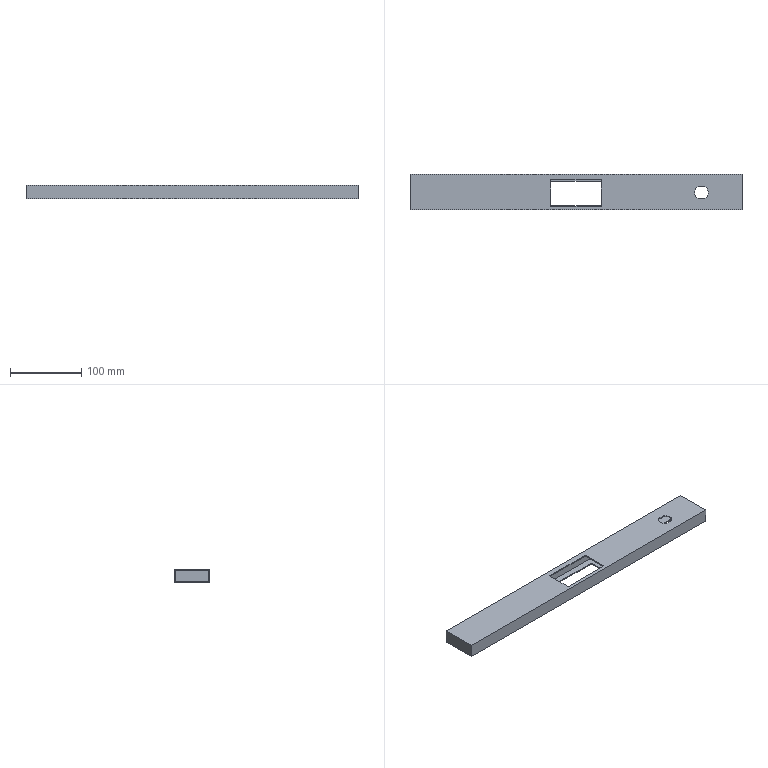Part | SolidWorks | features ICE 4, Extrusion 1, Shell 1 | 1 solid | 30 faces | box 466 x 50 x 19 mm | volume 83409 mm3 | plane 24 | cylinder 6 | commonest cylinder face diameters 19 x3 60 x3
STEP:
#1=CARTESIAN_POINT('',(379.,24.,1.5));
#2=VERTEX_POINT('',#1);
#3=CARTESIAN_POINT('',(381.728,36.5,1.5));
#4=VERTEX_POINT('',#3);
#5=CARTESIAN_POINT('',(409.,24.,1.5));
#6=DIRECTION('',(0.,0.,-1.));
#7=DIRECTION('',(-1.,0.,0.));
#8=AXIS2_PLACEMENT_3D('',#5,#6,#7);
#9=CIRCLE('',#8,30.);
#10=EDGE_CURVE('',#2,#4,#9,.T.);
#11=ORIENTED_EDGE('',*,*,#10,.F.);
#12=CARTESIAN_POINT('',(379.,24.,0.));
#13=VERTEX_POINT('',#12);
#14=CARTESIAN_POINT('',(379.,24.,2.));
#15=DIRECTION('',(0.,0.,-1.));
#16=VECTOR('',#15,1000.);
#17=LINE('',#14,#16);
#18=EDGE_CURVE('',#2,#13,#17,.T.);
#19=ORIENTED_EDGE('',*,*,#18,.T.);
#20=CARTESIAN_POINT('',(381.728,36.5,0.));
#21=VERTEX_POINT('',#20);
#22=CARTESIAN_POINT('',(409.,24.,0.));
#23=DIRECTION('',(0.,0.,-1.));
#24=DIRECTION('',(-1.,0.,0.));
#25=AXIS2_PLACEMENT_3D('',#22,#23,#24);
#26=CIRCLE('',#25,30.);
#27=EDGE_CURVE('',#13,#21,#26,.T.);
#28=ORIENTED_EDGE('',*,*,#27,.T.);
#29=CARTESIAN_POINT('',(381.728,36.5,2.));
#30=DIRECTION('',(0.,0.,-1.));
#31=VECTOR('',#30,1000.);
#32=LINE('',#29,#31);
#33=EDGE_CURVE('',#4,#21,#32,.T.);
#34=ORIENTED_EDGE('',*,*,#33,.F.);
#35=EDGE_LOOP('',(#11,#19,#28,#34));
#36=FACE_OUTER_BOUND('',#35,.T.);
#37=CARTESIAN_POINT('',(409.,24.,2.));
#38=DIRECTION('',(0.,0.,-1.));
#39=DIRECTION('',(-1.,0.,0.));
#40=AXIS2_PLACEMENT_3D('',#37,#38,#39);
#41=CYLINDRICAL_SURFACE('',#40,30.);
#42=ADVANCED_FACE('',(#36),#41,.F.);
#43=CARTESIAN_POINT('',(399.5,24.,19.));
#44=VERTEX_POINT('',#43);
#45=CARTESIAN_POINT('',(404.29,32.25,19.));
#46=VERTEX_POINT('',#45);
#47=CARTESIAN_POINT('',(409.,24.,19.));
#48=DIRECTION('',(0.,0.,-1.));
#49=DIRECTION('',(-1.,0.,0.));
#50=AXIS2_PLACEMENT_3D('',#47,#48,#49);
#51=CIRCLE('',#50,9.5);
#52=EDGE_CURVE('',#44,#46,#51,.T.);
#53=ORIENTED_EDGE('',*,*,#52,.F.);
#54=CARTESIAN_POINT('',(399.5,24.,17.5));
#55=VERTEX_POINT('',#54);
#56=CARTESIAN_POINT('',(399.5,24.,19.));
#57=DIRECTION('',(0.,0.,-1.));
#58=VECTOR('',#57,1000.);
#59=LINE('',#56,#58);
#60=EDGE_CURVE('',#44,#55,#59,.T.);
#61=ORIENTED_EDGE('',*,*,#60,.T.);
#62=CARTESIAN_POINT('',(404.29,32.25,17.5));
#63=VERTEX_POINT('',#62);
#64=CARTESIAN_POINT('',(409.,24.,17.5));
#65=DIRECTION('',(0.,0.,-1.));
#66=DIRECTION('',(-1.,0.,0.));
#67=AXIS2_PLACEMENT_3D('',#64,#65,#66);
#68=CIRCLE('',#67,9.5);
#69=EDGE_CURVE('',#55,#63,#68,.T.);
#70=ORIENTED_EDGE('',*,*,#69,.T.);
#71=CARTESIAN_POINT('',(404.29,32.25,19.));
#72=DIRECTION('',(0.,0.,-1.));
#73=VECTOR('',#72,1000.);
#74=LINE('',#71,#73);
#75=EDGE_CURVE('',#46,#63,#74,.T.);
#76=ORIENTED_EDGE('',*,*,#75,.F.);
#77=EDGE_LOOP('',(#53,#61,#70,#76));
#78=FACE_OUTER_BOUND('',#77,.T.);
#79=CARTESIAN_POINT('',(409.,24.,19.));
#80=DIRECTION('',(0.,0.,-1.));
#81=DIRECTION('',(-1.,0.,0.));
#82=AXIS2_PLACEMENT_3D('',#79,#80,#81);
#83=CYLINDRICAL_SURFACE('',#82,9.5);
#84=ADVANCED_FACE('',(#78),#83,.F.);
#85=CARTESIAN_POINT('',(0.,50.,0.));
#86=VERTEX_POINT('',#85);
#87=CARTESIAN_POINT('',(0.,0.,0.));
#88=VERTEX_POINT('',#87);
#89=CARTESIAN_POINT('',(0.,0.,0.));
#90=DIRECTION('',(0.,-1.,0.));
#91=VECTOR('',#90,1000.);
#92=LINE('',#89,#91);
#93=EDGE_CURVE('',#86,#88,#92,.T.);
#94=ORIENTED_EDGE('',*,*,#93,.T.);
#95=CARTESIAN_POINT('',(0.,0.,19.));
#96=VERTEX_POINT('',#95);
#97=CARTESIAN_POINT('',(0.,0.,19.));
#98=DIRECTION('',(0.,0.,-1.));
#99=VECTOR('',#98,1000.);
#100=LINE('',#97,#99);
#101=EDGE_CURVE('',#96,#88,#100,.T.);
#102=ORIENTED_EDGE('',*,*,#101,.F.);
#103=CARTESIAN_POINT('',(0.,50.,19.));
#104=VERTEX_POINT('',#103);
#105=CARTESIAN_POINT('',(0.,0.,19.));
#106=DIRECTION('',(0.,-1.,0.));
#107=VECTOR('',#106,1000.);
#108=LINE('',#105,#107);
#109=EDGE_CURVE('',#104,#96,#108,.T.);
#110=ORIENTED_EDGE('',*,*,#109,.F.);
#111=CARTESIAN_POINT('',(0.,50.,19.));
#112=DIRECTION('',(0.,0.,-1.));
#113=VECTOR('',#112,1000.);
#114=LINE('',#111,#113);
#115=EDGE_CURVE('',#104,#86,#114,.T.);
#116=ORIENTED_EDGE('',*,*,#115,.T.);
#117=EDGE_LOOP('',(#94,#102,#110,#116));
#118=FACE_OUTER_BOUND('',#117,.T.);
#119=CARTESIAN_POINT('',(0.,0.,19.));
#120=DIRECTION('',(1.,0.,0.));
#121=DIRECTION('',(0.,0.,-1.));
#122=AXIS2_PLACEMENT_3D('',#119,#120,#121);
#123=PLANE('',#122);
#124=ADVANCED_FACE('',(#118),#123,.F.);
#125=CARTESIAN_POINT('',(466.,0.,0.));
#126=VERTEX_POINT('',#125);
#127=CARTESIAN_POINT('',(0.,0.,0.));
#128=DIRECTION('',(1.,0.,0.));
#129=VECTOR('',#128,1000.);
#130=LINE('',#127,#129);
#131=EDGE_CURVE('',#88,#126,#130,.T.);
#132=ORIENTED_EDGE('',*,*,#131,.T.);
#133=CARTESIAN_POINT('',(466.,0.,19.));
#134=VERTEX_POINT('',#133);
#135=CARTESIAN_POINT('',(466.,0.,19.));
#136=DIRECTION('',(0.,0.,-1.));
#137=VECTOR('',#136,1000.);
#138=LINE('',#135,#137);
#139=EDGE_CURVE('',#134,#126,#138,.T.);
#140=ORIENTED_EDGE('',*,*,#139,.F.);
#141=CARTESIAN_POINT('',(0.,0.,19.));
#142=DIRECTION('',(1.,0.,0.));
#143=VECTOR('',#142,1000.);
#144=LINE('',#141,#143);
#145=EDGE_CURVE('',#96,#134,#144,.T.);
#146=ORIENTED_EDGE('',*,*,#145,.F.);
#147=ORIENTED_EDGE('',*,*,#101,.T.);
#148=EDGE_LOOP('',(#132,#140,#146,#147));
#149=FACE_OUTER_BOUND('',#148,.T.);
#150=CARTESIAN_POINT('',(0.,0.,19.));
#151=DIRECTION('',(0.,1.,0.));
#152=DIRECTION('',(0.,0.,1.));
#153=AXIS2_PLACEMENT_3D('',#150,#151,#152);
#154=PLANE('',#153);
#155=ADVANCED_FACE('',(#149),#154,.F.);
#156=CARTESIAN_POINT('',(466.,50.,0.));
#157=VERTEX_POINT('',#156);
#158=CARTESIAN_POINT('',(466.,0.,0.));
#159=DIRECTION('',(0.,1.,0.));
#160=VECTOR('',#159,1000.);
#161=LINE('',#158,#160);
#162=EDGE_CURVE('',#126,#157,#161,.T.);
#163=ORIENTED_EDGE('',*,*,#162,.T.);
#164=CARTESIAN_POINT('',(466.,50.,19.));
#165=VERTEX_POINT('',#164);
#166=CARTESIAN_POINT('',(466.,50.,19.));
#167=DIRECTION('',(0.,0.,-1.));
#168=VECTOR('',#167,1000.);
#169=LINE('',#166,#168);
#170=EDGE_CURVE('',#165,#157,#169,.T.);
#171=ORIENTED_EDGE('',*,*,#170,.F.);
#172=CARTESIAN_POINT('',(466.,0.,19.));
#173=DIRECTION('',(0.,1.,0.));
#174=VECTOR('',#173,1000.);
#175=LINE('',#172,#174);
#176=EDGE_CURVE('',#134,#165,#175,.T.);
#177=ORIENTED_EDGE('',*,*,#176,.F.);
#178=ORIENTED_EDGE('',*,*,#139,.T.);
#179=EDGE_LOOP('',(#163,#171,#177,#178));
#180=FACE_OUTER_BOUND('',#179,.T.);
#181=CARTESIAN_POINT('',(466.,0.,19.));
#182=DIRECTION('',(-1.,0.,0.));
#183=DIRECTION('',(0.,0.,1.));
#184=AXIS2_PLACEMENT_3D('',#181,#182,#183);
#185=PLANE('',#184);
#186=ADVANCED_FACE('',(#180),#185,.F.);
#187=CARTESIAN_POINT('',(0.,50.,0.));
#188=DIRECTION('',(-1.,0.,0.));
#189=VECTOR('',#188,1000.);
#190=LINE('',#187,#189);
#191=EDGE_CURVE('',#157,#86,#190,.T.);
#192=ORIENTED_EDGE('',*,*,#191,.T.);
#193=ORIENTED_EDGE('',*,*,#115,.F.);
#194=CARTESIAN_POINT('',(0.,50.,19.));
#195=DIRECTION('',(-1.,0.,0.));
#196=VECTOR('',#195,1000.);
#197=LINE('',#194,#196);
#198=EDGE_CURVE('',#165,#104,#197,.T.);
#199=ORIENTED_EDGE('',*,*,#198,.F.);
#200=ORIENTED_EDGE('',*,*,#170,.T.);
#201=EDGE_LOOP('',(#192,#193,#199,#200));
#202=FACE_OUTER_BOUND('',#201,.T.);
#203=CARTESIAN_POINT('',(0.,50.,19.));
#204=DIRECTION('',(0.,-1.,0.));
#205=DIRECTION('',(0.,0.,-1.));
#206=AXIS2_PLACEMENT_3D('',#203,#204,#205);
#207=PLANE('',#206);
#208=ADVANCED_FACE('',(#202),#207,.F.);
#209=CARTESIAN_POINT('',(413.71,32.25,19.));
#210=VERTEX_POINT('',#209);
#211=CARTESIAN_POINT('',(413.71,32.25,19.));
#212=DIRECTION('',(1.,0.,0.));
#213=VECTOR('',#212,1000.);
#214=LINE('',#211,#213);
#215=EDGE_CURVE('',#46,#210,#214,.T.);
#216=ORIENTED_EDGE('',*,*,#215,.T.);
#217=CARTESIAN_POINT('',(413.71,15.75,19.));
#218=VERTEX_POINT('',#217);
#219=CARTESIAN_POINT('',(409.,24.,19.));
#220=DIRECTION('',(0.,0.,-1.));
#221=DIRECTION('',(-1.,0.,0.));
#222=AXIS2_PLACEMENT_3D('',#219,#220,#221);
#223=CIRCLE('',#222,9.5);
#224=EDGE_CURVE('',#210,#218,#223,.T.);
#225=ORIENTED_EDGE('',*,*,#224,.T.);
#226=CARTESIAN_POINT('',(404.29,15.75,19.));
#227=VERTEX_POINT('',#226);
#228=CARTESIAN_POINT('',(413.71,15.75,19.));
#229=DIRECTION('',(-1.,0.,0.));
#230=VECTOR('',#229,1000.);
#231=LINE('',#228,#230);
#232=EDGE_CURVE('',#218,#227,#231,.T.);
#233=ORIENTED_EDGE('',*,*,#232,.T.);
#234=CARTESIAN_POINT('',(409.,24.,19.));
#235=DIRECTION('',(0.,0.,-1.));
#236=DIRECTION('',(-1.,0.,0.));
#237=AXIS2_PLACEMENT_3D('',#234,#235,#236);
#238=CIRCLE('',#237,9.5);
#239=EDGE_CURVE('',#227,#44,#238,.T.);
#240=ORIENTED_EDGE('',*,*,#239,.T.);
#241=ORIENTED_EDGE('',*,*,#52,.T.);
#242=EDGE_LOOP('',(#216,#225,#233,#240,#241));
#243=FACE_BOUND('',#242,.T.);
#244=CARTESIAN_POINT('',(197.5,5.,19.));
#245=VERTEX_POINT('',#244);
#246=CARTESIAN_POINT('',(268.5,5.,19.));
#247=VERTEX_POINT('',#246);
#248=CARTESIAN_POINT('',(197.5,5.,19.));
#249=DIRECTION('',(1.,0.,0.));
#250=VECTOR('',#249,1000.);
#251=LINE('',#248,#250);
#252=EDGE_CURVE('',#245,#247,#251,.T.);
#253=ORIENTED_EDGE('',*,*,#252,.F.);
#254=CARTESIAN_POINT('',(197.5,42.,19.));
#255=VERTEX_POINT('',#254);
#256=CARTESIAN_POINT('',(197.5,5.,19.));
#257=DIRECTION('',(0.,-1.,0.));
#258=VECTOR('',#257,1000.);
#259=LINE('',#256,#258);
#260=EDGE_CURVE('',#255,#245,#259,.T.);
#261=ORIENTED_EDGE('',*,*,#260,.F.);
#262=CARTESIAN_POINT('',(268.5,42.,19.));
#263=VERTEX_POINT('',#262);
#264=CARTESIAN_POINT('',(197.5,42.,19.));
#265=DIRECTION('',(-1.,0.,0.));
#266=VECTOR('',#265,1000.);
#267=LINE('',#264,#266);
#268=EDGE_CURVE('',#263,#255,#267,.T.);
#269=ORIENTED_EDGE('',*,*,#268,.F.);
#270=CARTESIAN_POINT('',(268.5,5.,19.));
#271=DIRECTION('',(0.,1.,0.));
#272=VECTOR('',#271,1000.);
#273=LINE('',#270,#272);
#274=EDGE_CURVE('',#247,#263,#273,.T.);
#275=ORIENTED_EDGE('',*,*,#274,.F.);
#276=EDGE_LOOP('',(#253,#261,#269,#275));
#277=FACE_BOUND('',#276,.T.);
#278=ORIENTED_EDGE('',*,*,#109,.T.);
#279=ORIENTED_EDGE('',*,*,#145,.T.);
#280=ORIENTED_EDGE('',*,*,#176,.T.);
#281=ORIENTED_EDGE('',*,*,#198,.T.);
#282=EDGE_LOOP('',(#278,#279,#280,#281));
#283=FACE_OUTER_BOUND('',#282,.T.);
#284=CARTESIAN_POINT('',(0.,50.,19.));
#285=DIRECTION('',(0.,0.,-1.));
#286=DIRECTION('',(-1.,0.,0.));
#287=AXIS2_PLACEMENT_3D('',#284,#285,#286);
#288=PLANE('',#287);
#289=ADVANCED_FACE('',(#243,#277,#283),#288,.F.);
#290=CARTESIAN_POINT('',(381.728,11.5,0.));
#291=VERTEX_POINT('',#290);
#292=CARTESIAN_POINT('',(409.,24.,0.));
#293=DIRECTION('',(0.,0.,-1.));
#294=DIRECTION('',(-1.,0.,0.));
#295=AXIS2_PLACEMENT_3D('',#292,#293,#294);
#296=CIRCLE('',#295,30.);
#297=EDGE_CURVE('',#291,#13,#296,.T.);
#298=ORIENTED_EDGE('',*,*,#297,.F.);
#299=CARTESIAN_POINT('',(436.272,11.5,0.));
#300=VERTEX_POINT('',#299);
#301=CARTESIAN_POINT('',(436.272,11.5,0.));
#302=DIRECTION('',(-1.,0.,0.));
#303=VECTOR('',#302,1000.);
#304=LINE('',#301,#303);
#305=EDGE_CURVE('',#300,#291,#304,.T.);
#306=ORIENTED_EDGE('',*,*,#305,.F.);
#307=CARTESIAN_POINT('',(436.272,36.5,0.));
#308=VERTEX_POINT('',#307);
#309=CARTESIAN_POINT('',(409.,24.,0.));
#310=DIRECTION('',(0.,0.,-1.));
#311=DIRECTION('',(-1.,0.,0.));
#312=AXIS2_PLACEMENT_3D('',#309,#310,#311);
#313=CIRCLE('',#312,30.);
#314=EDGE_CURVE('',#308,#300,#313,.T.);
#315=ORIENTED_EDGE('',*,*,#314,.F.);
#316=CARTESIAN_POINT('',(436.272,36.5,0.));
#317=DIRECTION('',(1.,0.,0.));
#318=VECTOR('',#317,1000.);
#319=LINE('',#316,#318);
#320=EDGE_CURVE('',#21,#308,#319,.T.);
#321=ORIENTED_EDGE('',*,*,#320,.F.);
#322=ORIENTED_EDGE('',*,*,#27,.F.);
#323=EDGE_LOOP('',(#298,#306,#315,#321,#322));
#324=FACE_BOUND('',#323,.T.);
#325=CARTESIAN_POINT('',(278.,40.,0.));
#326=VERTEX_POINT('',#325);
#327=CARTESIAN_POINT('',(278.,6.,0.));
#328=VERTEX_POINT('',#327);
#329=CARTESIAN_POINT('',(278.,6.,0.));
#330=DIRECTION('',(0.,-1.,0.));
#331=VECTOR('',#330,1000.);
#332=LINE('',#329,#331);
#333=EDGE_CURVE('',#326,#328,#332,.T.);
#334=ORIENTED_EDGE('',*,*,#333,.F.);
#335=CARTESIAN_POINT('',(188.,40.,0.));
#336=VERTEX_POINT('',#335);
#337=CARTESIAN_POINT('',(278.,40.,0.));
#338=DIRECTION('',(1.,0.,0.));
#339=VECTOR('',#338,1000.);
#340=LINE('',#337,#339);
#341=EDGE_CURVE('',#336,#326,#340,.T.);
#342=ORIENTED_EDGE('',*,*,#341,.F.);
#343=CARTESIAN_POINT('',(188.,6.,0.));
#344=VERTEX_POINT('',#343);
#345=CARTESIAN_POINT('',(188.,6.,0.));
#346=DIRECTION('',(0.,1.,0.));
#347=VECTOR('',#346,1000.);
#348=LINE('',#345,#347);
#349=EDGE_CURVE('',#344,#336,#348,.T.);
#350=ORIENTED_EDGE('',*,*,#349,.F.);
#351=CARTESIAN_POINT('',(278.,6.,0.));
#352=DIRECTION('',(-1.,0.,0.));
#353=VECTOR('',#352,1000.);
#354=LINE('',#351,#353);
#355=EDGE_CURVE('',#328,#344,#354,.T.);
#356=ORIENTED_EDGE('',*,*,#355,.F.);
#357=EDGE_LOOP('',(#334,#342,#350,#356));
#358=FACE_BOUND('',#357,.T.);
#359=ORIENTED_EDGE('',*,*,#93,.F.);
#360=ORIENTED_EDGE('',*,*,#191,.F.);
#361=ORIENTED_EDGE('',*,*,#162,.F.);
#362=ORIENTED_EDGE('',*,*,#131,.F.);
#363=EDGE_LOOP('',(#359,#360,#361,#362));
#364=FACE_OUTER_BOUND('',#363,.T.);
#365=CARTESIAN_POINT('',(0.,50.,0.));
#366=DIRECTION('',(0.,0.,-1.));
#367=DIRECTION('',(-1.,0.,0.));
#368=AXIS2_PLACEMENT_3D('',#365,#366,#367);
#369=PLANE('',#368);
#370=ADVANCED_FACE('',(#324,#358,#364),#369,.T.);
#371=ORIENTED_EDGE('',*,*,#260,.T.);
#372=CARTESIAN_POINT('',(197.5,5.,17.5));
#373=VERTEX_POINT('',#372);
#374=CARTESIAN_POINT('',(197.5,5.,17.5));
#375=DIRECTION('',(0.,0.,1.));
#376=VECTOR('',#375,1000.);
#377=LINE('',#374,#376);
#378=EDGE_CURVE('',#373,#245,#377,.T.);
#379=ORIENTED_EDGE('',*,*,#378,.F.);
#380=CARTESIAN_POINT('',(197.5,42.,17.5));
#381=VERTEX_POINT('',#380);
#382=CARTESIAN_POINT('',(197.5,5.,17.5));
#383=DIRECTION('',(0.,-1.,0.));
#384=VECTOR('',#383,1000.);
#385=LINE('',#382,#384);
#386=EDGE_CURVE('',#381,#373,#385,.T.);
#387=ORIENTED_EDGE('',*,*,#386,.F.);
#388=CARTESIAN_POINT('',(197.5,42.,17.5));
#389=DIRECTION('',(0.,0.,1.));
#390=VECTOR('',#389,1000.);
#391=LINE('',#388,#390);
#392=EDGE_CURVE('',#381,#255,#391,.T.);
#393=ORIENTED_EDGE('',*,*,#392,.T.);
#394=EDGE_LOOP('',(#371,#379,#387,#393));
#395=FACE_OUTER_BOUND('',#394,.T.);
#396=CARTESIAN_POINT('',(197.5,5.,17.5));
#397=DIRECTION('',(-1.,0.,0.));
#398=DIRECTION('',(0.,-1.,0.));
#399=AXIS2_PLACEMENT_3D('',#396,#397,#398);
#400=PLANE('',#399);
#401=ADVANCED_FACE('',(#395),#400,.F.);
#402=ORIENTED_EDGE('',*,*,#268,.T.);
#403=ORIENTED_EDGE('',*,*,#392,.F.);
#404=CARTESIAN_POINT('',(268.5,42.,17.5));
#405=VERTEX_POINT('',#404);
#406=CARTESIAN_POINT('',(197.5,42.,17.5));
#407=DIRECTION('',(-1.,0.,0.));
#408=VECTOR('',#407,1000.);
#409=LINE('',#406,#408);
#410=EDGE_CURVE('',#405,#381,#409,.T.);
#411=ORIENTED_EDGE('',*,*,#410,.F.);
#412=CARTESIAN_POINT('',(268.5,42.,17.5));
#413=DIRECTION('',(0.,0.,1.));
#414=VECTOR('',#413,1000.);
#415=LINE('',#412,#414);
#416=EDGE_CURVE('',#405,#263,#415,.T.);
#417=ORIENTED_EDGE('',*,*,#416,.T.);
#418=EDGE_LOOP('',(#402,#403,#411,#417));
#419=FACE_OUTER_BOUND('',#418,.T.);
#420=CARTESIAN_POINT('',(197.5,42.,17.5));
#421=DIRECTION('',(0.,1.,0.));
#422=DIRECTION('',(-1.,0.,0.));
#423=AXIS2_PLACEMENT_3D('',#420,#421,#422);
#424=PLANE('',#423);
#425=ADVANCED_FACE('',(#419),#424,.F.);
#426=ORIENTED_EDGE('',*,*,#274,.T.);
#427=ORIENTED_EDGE('',*,*,#416,.F.);
#428=CARTESIAN_POINT('',(268.5,5.,17.5));
#429=VERTEX_POINT('',#428);
#430=CARTESIAN_POINT('',(268.5,5.,17.5));
#431=DIRECTION('',(0.,1.,0.));
#432=VECTOR('',#431,1000.);
#433=LINE('',#430,#432);
#434=EDGE_CURVE('',#429,#405,#433,.T.);
#435=ORIENTED_EDGE('',*,*,#434,.F.);
#436=CARTESIAN_POINT('',(268.5,5.,17.5));
#437=DIRECTION('',(0.,0.,1.));
#438=VECTOR('',#437,1000.);
#439=LINE('',#436,#438);
#440=EDGE_CURVE('',#429,#247,#439,.T.);
#441=ORIENTED_EDGE('',*,*,#440,.T.);
#442=EDGE_LOOP('',(#426,#427,#435,#441));
#443=FACE_OUTER_BOUND('',#442,.T.);
#444=CARTESIAN_POINT('',(268.5,5.,17.5));
#445=DIRECTION('',(1.,0.,0.));
#446=DIRECTION('',(0.,1.,0.));
#447=AXIS2_PLACEMENT_3D('',#444,#445,#446);
#448=PLANE('',#447);
#449=ADVANCED_FACE('',(#443),#448,.F.);
#450=ORIENTED_EDGE('',*,*,#252,.T.);
#451=ORIENTED_EDGE('',*,*,#440,.F.);
#452=CARTESIAN_POINT('',(197.5,5.,17.5));
#453=DIRECTION('',(1.,0.,0.));
#454=VECTOR('',#453,1000.);
#455=LINE('',#452,#454);
#456=EDGE_CURVE('',#373,#429,#455,.T.);
#457=ORIENTED_EDGE('',*,*,#456,.F.);
#458=ORIENTED_EDGE('',*,*,#378,.T.);
#459=EDGE_LOOP('',(#450,#451,#457,#458));
#460=FACE_OUTER_BOUND('',#459,.T.);
#461=CARTESIAN_POINT('',(197.5,5.,17.5));
#462=DIRECTION('',(0.,-1.,0.));
#463=DIRECTION('',(1.,0.,0.));
#464=AXIS2_PLACEMENT_3D('',#461,#462,#463);
#465=PLANE('',#464);
#466=ADVANCED_FACE('',(#460),#465,.F.);
#467=CARTESIAN_POINT('',(413.71,32.25,17.5));
#468=VERTEX_POINT('',#467);
#469=CARTESIAN_POINT('',(413.71,15.75,17.5));
#470=VERTEX_POINT('',#469);
#471=CARTESIAN_POINT('',(409.,24.,17.5));
#472=DIRECTION('',(0.,0.,-1.));
#473=DIRECTION('',(-1.,0.,0.));
#474=AXIS2_PLACEMENT_3D('',#471,#472,#473);
#475=CIRCLE('',#474,9.5);
#476=EDGE_CURVE('',#468,#470,#475,.T.);
#477=ORIENTED_EDGE('',*,*,#476,.F.);
#478=CARTESIAN_POINT('',(0.,32.25,17.5));
#479=DIRECTION('',(1.,0.,0.));
#480=VECTOR('',#479,1000.);
#481=LINE('',#478,#480);
#482=EDGE_CURVE('',#63,#468,#481,.T.);
#483=ORIENTED_EDGE('',*,*,#482,.F.);
#484=ORIENTED_EDGE('',*,*,#69,.F.);
#485=CARTESIAN_POINT('',(404.29,15.75,17.5));
#486=VERTEX_POINT('',#485);
#487=CARTESIAN_POINT('',(409.,24.,17.5));
#488=DIRECTION('',(0.,0.,-1.));
#489=DIRECTION('',(-1.,0.,0.));
#490=AXIS2_PLACEMENT_3D('',#487,#488,#489);
#491=CIRCLE('',#490,9.5);
#492=EDGE_CURVE('',#486,#55,#491,.T.);
#493=ORIENTED_EDGE('',*,*,#492,.F.);
#494=CARTESIAN_POINT('',(0.,15.75,17.5));
#495=DIRECTION('',(-1.,0.,0.));
#496=VECTOR('',#495,1000.);
#497=LINE('',#494,#496);
#498=EDGE_CURVE('',#470,#486,#497,.T.);
#499=ORIENTED_EDGE('',*,*,#498,.F.);
#500=EDGE_LOOP('',(#477,#483,#484,#493,#499));
#501=FACE_BOUND('',#500,.T.);
#502=CARTESIAN_POINT('',(1.5,48.5,17.5));
#503=VERTEX_POINT('',#502);
#504=CARTESIAN_POINT('',(1.5,1.5,17.5));
#505=VERTEX_POINT('',#504);
#506=CARTESIAN_POINT('',(1.5,50.,17.5));
#507=DIRECTION('',(0.,-1.,0.));
#508=VECTOR('',#507,1000.);
#509=LINE('',#506,#508);
#510=EDGE_CURVE('',#503,#505,#509,.T.);
#511=ORIENTED_EDGE('',*,*,#510,.F.);
#512=CARTESIAN_POINT('',(464.5,48.5,17.5));
#513=VERTEX_POINT('',#512);
#514=CARTESIAN_POINT('',(0.,48.5,17.5));
#515=DIRECTION('',(-1.,0.,0.));
#516=VECTOR('',#515,1000.);
#517=LINE('',#514,#516);
#518=EDGE_CURVE('',#513,#503,#517,.T.);
#519=ORIENTED_EDGE('',*,*,#518,.F.);
#520=CARTESIAN_POINT('',(464.5,1.5,17.5));
#521=VERTEX_POINT('',#520);
#522=CARTESIAN_POINT('',(464.5,50.,17.5));
#523=DIRECTION('',(0.,1.,0.));
#524=VECTOR('',#523,1000.);
#525=LINE('',#522,#524);
#526=EDGE_CURVE('',#521,#513,#525,.T.);
#527=ORIENTED_EDGE('',*,*,#526,.F.);
#528=CARTESIAN_POINT('',(0.,1.5,17.5));
#529=DIRECTION('',(1.,0.,0.));
#530=VECTOR('',#529,1000.);
#531=LINE('',#528,#530);
#532=EDGE_CURVE('',#505,#521,#531,.T.);
#533=ORIENTED_EDGE('',*,*,#532,.F.);
#534=EDGE_LOOP('',(#511,#519,#527,#533));
#535=FACE_OUTER_BOUND('',#534,.T.);
#536=ORIENTED_EDGE('',*,*,#386,.T.);
#537=ORIENTED_EDGE('',*,*,#456,.T.);
#538=ORIENTED_EDGE('',*,*,#434,.T.);
#539=ORIENTED_EDGE('',*,*,#410,.T.);
#540=EDGE_LOOP('',(#536,#537,#538,#539));
#541=FACE_BOUND('',#540,.T.);
#542=CARTESIAN_POINT('',(0.,50.,17.5));
#543=DIRECTION('',(0.,0.,-1.));
#544=DIRECTION('',(-1.,0.,0.));
#545=AXIS2_PLACEMENT_3D('',#542,#543,#544);
#546=PLANE('',#545);
#547=ADVANCED_FACE('',(#501,#535,#541),#546,.T.);
#548=CARTESIAN_POINT('',(1.5,48.5,1.5));
#549=VERTEX_POINT('',#548);
#550=CARTESIAN_POINT('',(1.5,1.5,1.5));
#551=VERTEX_POINT('',#550);
#552=CARTESIAN_POINT('',(1.5,50.,1.5));
#553=DIRECTION('',(0.,-1.,0.));
#554=VECTOR('',#553,1000.);
#555=LINE('',#552,#554);
#556=EDGE_CURVE('',#549,#551,#555,.T.);
#557=ORIENTED_EDGE('',*,*,#556,.F.);
#558=CARTESIAN_POINT('',(1.5,48.5,19.));
#559=DIRECTION('',(0.,0.,-1.));
#560=VECTOR('',#559,1000.);
#561=LINE('',#558,#560);
#562=EDGE_CURVE('',#503,#549,#561,.T.);
#563=ORIENTED_EDGE('',*,*,#562,.F.);
#564=ORIENTED_EDGE('',*,*,#510,.T.);
#565=CARTESIAN_POINT('',(1.5,1.5,19.));
#566=DIRECTION('',(0.,0.,-1.));
#567=VECTOR('',#566,1000.);
#568=LINE('',#565,#567);
#569=EDGE_CURVE('',#505,#551,#568,.T.);
#570=ORIENTED_EDGE('',*,*,#569,.T.);
#571=EDGE_LOOP('',(#557,#563,#564,#570));
#572=FACE_OUTER_BOUND('',#571,.T.);
#573=CARTESIAN_POINT('',(1.5,0.,19.));
#574=DIRECTION('',(1.,0.,0.));
#575=DIRECTION('',(0.,0.,-1.));
#576=AXIS2_PLACEMENT_3D('',#573,#574,#575);
#577=PLANE('',#576);
#578=ADVANCED_FACE('',(#572),#577,.T.);
#579=CARTESIAN_POINT('',(464.5,1.5,1.5));
#580=VERTEX_POINT('',#579);
#581=CARTESIAN_POINT('',(0.,1.5,1.5));
#582=DIRECTION('',(1.,0.,0.));
#583=VECTOR('',#582,1000.);
#584=LINE('',#581,#583);
#585=EDGE_CURVE('',#551,#580,#584,.T.);
#586=ORIENTED_EDGE('',*,*,#585,.F.);
#587=ORIENTED_EDGE('',*,*,#569,.F.);
#588=ORIENTED_EDGE('',*,*,#532,.T.);
#589=CARTESIAN_POINT('',(464.5,1.5,19.));
#590=DIRECTION('',(0.,0.,-1.));
#591=VECTOR('',#590,1000.);
#592=LINE('',#589,#591);
#593=EDGE_CURVE('',#521,#580,#592,.T.);
#594=ORIENTED_EDGE('',*,*,#593,.T.);
#595=EDGE_LOOP('',(#586,#587,#588,#594));
#596=FACE_OUTER_BOUND('',#595,.T.);
#597=CARTESIAN_POINT('',(0.,1.5,19.));
#598=DIRECTION('',(0.,1.,0.));
#599=DIRECTION('',(0.,0.,1.));
#600=AXIS2_PLACEMENT_3D('',#597,#598,#599);
#601=PLANE('',#600);
#602=ADVANCED_FACE('',(#596),#601,.T.);
#603=CARTESIAN_POINT('',(464.5,48.5,1.5));
#604=VERTEX_POINT('',#603);
#605=CARTESIAN_POINT('',(464.5,50.,1.5));
#606=DIRECTION('',(0.,1.,0.));
#607=VECTOR('',#606,1000.);
#608=LINE('',#605,#607);
#609=EDGE_CURVE('',#580,#604,#608,.T.);
#610=ORIENTED_EDGE('',*,*,#609,.F.);
#611=ORIENTED_EDGE('',*,*,#593,.F.);
#612=ORIENTED_EDGE('',*,*,#526,.T.);
#613=CARTESIAN_POINT('',(464.5,48.5,19.));
#614=DIRECTION('',(0.,0.,-1.));
#615=VECTOR('',#614,1000.);
#616=LINE('',#613,#615);
#617=EDGE_CURVE('',#513,#604,#616,.T.);
#618=ORIENTED_EDGE('',*,*,#617,.T.);
#619=EDGE_LOOP('',(#610,#611,#612,#618));
#620=FACE_OUTER_BOUND('',#619,.T.);
#621=CARTESIAN_POINT('',(464.5,0.,19.));
#622=DIRECTION('',(-1.,0.,0.));
#623=DIRECTION('',(0.,0.,1.));
#624=AXIS2_PLACEMENT_3D('',#621,#622,#623);
#625=PLANE('',#624);
#626=ADVANCED_FACE('',(#620),#625,.T.);
#627=CARTESIAN_POINT('',(0.,48.5,1.5));
#628=DIRECTION('',(-1.,0.,0.));
#629=VECTOR('',#628,1000.);
#630=LINE('',#627,#629);
#631=EDGE_CURVE('',#604,#549,#630,.T.);
#632=ORIENTED_EDGE('',*,*,#631,.F.);
#633=ORIENTED_EDGE('',*,*,#617,.F.);
#634=ORIENTED_EDGE('',*,*,#518,.T.);
#635=ORIENTED_EDGE('',*,*,#562,.T.);
#636=EDGE_LOOP('',(#632,#633,#634,#635));
#637=FACE_OUTER_BOUND('',#636,.T.);
#638=CARTESIAN_POINT('',(0.,48.5,19.));
#639=DIRECTION('',(0.,-1.,0.));
#640=DIRECTION('',(0.,0.,-1.));
#641=AXIS2_PLACEMENT_3D('',#638,#639,#640);
#642=PLANE('',#641);
#643=ADVANCED_FACE('',(#637),#642,.T.);
#644=CARTESIAN_POINT('',(436.272,11.5,1.5));
#645=VERTEX_POINT('',#644);
#646=CARTESIAN_POINT('',(381.728,11.5,1.5));
#647=VERTEX_POINT('',#646);
#648=CARTESIAN_POINT('',(0.,11.5,1.5));
#649=DIRECTION('',(-1.,0.,0.));
#650=VECTOR('',#649,1000.);
#651=LINE('',#648,#650);
#652=EDGE_CURVE('',#645,#647,#651,.T.);
#653=ORIENTED_EDGE('',*,*,#652,.T.);
#654=CARTESIAN_POINT('',(409.,24.,1.5));
#655=DIRECTION('',(0.,0.,-1.));
#656=DIRECTION('',(-1.,0.,0.));
#657=AXIS2_PLACEMENT_3D('',#654,#655,#656);
#658=CIRCLE('',#657,30.);
#659=EDGE_CURVE('',#647,#2,#658,.T.);
#660=ORIENTED_EDGE('',*,*,#659,.T.);
#661=ORIENTED_EDGE('',*,*,#10,.T.);
#662=CARTESIAN_POINT('',(436.272,36.5,1.5));
#663=VERTEX_POINT('',#662);
#664=CARTESIAN_POINT('',(0.,36.5,1.5));
#665=DIRECTION('',(1.,0.,0.));
#666=VECTOR('',#665,1000.);
#667=LINE('',#664,#666);
#668=EDGE_CURVE('',#4,#663,#667,.T.);
#669=ORIENTED_EDGE('',*,*,#668,.T.);
#670=CARTESIAN_POINT('',(409.,24.,1.5));
#671=DIRECTION('',(0.,0.,-1.));
#672=DIRECTION('',(-1.,0.,0.));
#673=AXIS2_PLACEMENT_3D('',#670,#671,#672);
#674=CIRCLE('',#673,30.);
#675=EDGE_CURVE('',#663,#645,#674,.T.);
#676=ORIENTED_EDGE('',*,*,#675,.T.);
#677=EDGE_LOOP('',(#653,#660,#661,#669,#676));
#678=FACE_BOUND('',#677,.T.);
#679=CARTESIAN_POINT('',(188.,40.,1.5));
#680=VERTEX_POINT('',#679);
#681=CARTESIAN_POINT('',(278.,40.,1.5));
#682=VERTEX_POINT('',#681);
#683=CARTESIAN_POINT('',(278.,40.,1.5));
#684=DIRECTION('',(1.,0.,0.));
#685=VECTOR('',#684,1000.);
#686=LINE('',#683,#685);
#687=EDGE_CURVE('',#680,#682,#686,.T.);
#688=ORIENTED_EDGE('',*,*,#687,.T.);
#689=CARTESIAN_POINT('',(278.,6.,1.5));
#690=VERTEX_POINT('',#689);
#691=CARTESIAN_POINT('',(278.,6.,1.5));
#692=DIRECTION('',(0.,-1.,0.));
#693=VECTOR('',#692,1000.);
#694=LINE('',#691,#693);
#695=EDGE_CURVE('',#682,#690,#694,.T.);
#696=ORIENTED_EDGE('',*,*,#695,.T.);
#697=CARTESIAN_POINT('',(188.,6.,1.5));
#698=VERTEX_POINT('',#697);
#699=CARTESIAN_POINT('',(278.,6.,1.5));
#700=DIRECTION('',(-1.,0.,0.));
#701=VECTOR('',#700,1000.);
#702=LINE('',#699,#701);
#703=EDGE_CURVE('',#690,#698,#702,.T.);
#704=ORIENTED_EDGE('',*,*,#703,.T.);
#705=CARTESIAN_POINT('',(188.,6.,1.5));
#706=DIRECTION('',(0.,1.,0.));
#707=VECTOR('',#706,1000.);
#708=LINE('',#705,#707);
#709=EDGE_CURVE('',#698,#680,#708,.T.);
#710=ORIENTED_EDGE('',*,*,#709,.T.);
#711=EDGE_LOOP('',(#688,#696,#704,#710));
#712=FACE_BOUND('',#711,.T.);
#713=ORIENTED_EDGE('',*,*,#556,.T.);
#714=ORIENTED_EDGE('',*,*,#585,.T.);
#715=ORIENTED_EDGE('',*,*,#609,.T.);
#716=ORIENTED_EDGE('',*,*,#631,.T.);
#717=EDGE_LOOP('',(#713,#714,#715,#716));
#718=FACE_OUTER_BOUND('',#717,.T.);
#719=CARTESIAN_POINT('',(0.,50.,1.5));
#720=DIRECTION('',(0.,0.,-1.));
#721=DIRECTION('',(-1.,0.,0.));
#722=AXIS2_PLACEMENT_3D('',#719,#720,#721);
#723=PLANE('',#722);
#724=ADVANCED_FACE('',(#678,#712,#718),#723,.F.);
#725=ORIENTED_EDGE('',*,*,#333,.T.);
#726=CARTESIAN_POINT('',(278.,6.,1.5));
#727=DIRECTION('',(0.,0.,-1.));
#728=VECTOR('',#727,1000.);
#729=LINE('',#726,#728);
#730=EDGE_CURVE('',#690,#328,#729,.T.);
#731=ORIENTED_EDGE('',*,*,#730,.F.);
#732=ORIENTED_EDGE('',*,*,#695,.F.);
#733=CARTESIAN_POINT('',(278.,40.,1.5));
#734=DIRECTION('',(0.,0.,-1.));
#735=VECTOR('',#734,1000.);
#736=LINE('',#733,#735);
#737=EDGE_CURVE('',#682,#326,#736,.T.);
#738=ORIENTED_EDGE('',*,*,#737,.T.);
#739=EDGE_LOOP('',(#725,#731,#732,#738));
#740=FACE_OUTER_BOUND('',#739,.T.);
#741=CARTESIAN_POINT('',(278.,6.,1.5));
#742=DIRECTION('',(1.,0.,0.));
#743=DIRECTION('',(0.,0.,-1.));
#744=AXIS2_PLACEMENT_3D('',#741,#742,#743);
#745=PLANE('',#744);
#746=ADVANCED_FACE('',(#740),#745,.F.);
#747=ORIENTED_EDGE('',*,*,#341,.T.);
#748=ORIENTED_EDGE('',*,*,#737,.F.);
#749=ORIENTED_EDGE('',*,*,#687,.F.);
#750=CARTESIAN_POINT('',(188.,40.,1.5));
#751=DIRECTION('',(0.,0.,-1.));
#752=VECTOR('',#751,1000.);
#753=LINE('',#750,#752);
#754=EDGE_CURVE('',#680,#336,#753,.T.);
#755=ORIENTED_EDGE('',*,*,#754,.T.);
#756=EDGE_LOOP('',(#747,#748,#749,#755));
#757=FACE_OUTER_BOUND('',#756,.T.);
#758=CARTESIAN_POINT('',(278.,40.,1.5));
#759=DIRECTION('',(0.,1.,0.));
#760=DIRECTION('',(-1.,0.,0.));
#761=AXIS2_PLACEMENT_3D('',#758,#759,#760);
#762=PLANE('',#761);
#763=ADVANCED_FACE('',(#757),#762,.F.);
#764=ORIENTED_EDGE('',*,*,#349,.T.);
#765=ORIENTED_EDGE('',*,*,#754,.F.);
#766=ORIENTED_EDGE('',*,*,#709,.F.);
#767=CARTESIAN_POINT('',(188.,6.,1.5));
#768=DIRECTION('',(0.,0.,-1.));
#769=VECTOR('',#768,1000.);
#770=LINE('',#767,#769);
#771=EDGE_CURVE('',#698,#344,#770,.T.);
#772=ORIENTED_EDGE('',*,*,#771,.T.);
#773=EDGE_LOOP('',(#764,#765,#766,#772));
#774=FACE_OUTER_BOUND('',#773,.T.);
#775=CARTESIAN_POINT('',(188.,6.,1.5));
#776=DIRECTION('',(-1.,0.,0.));
#777=DIRECTION('',(0.,0.,1.));
#778=AXIS2_PLACEMENT_3D('',#775,#776,#777);
#779=PLANE('',#778);
#780=ADVANCED_FACE('',(#774),#779,.F.);
#781=ORIENTED_EDGE('',*,*,#355,.T.);
#782=ORIENTED_EDGE('',*,*,#771,.F.);
#783=ORIENTED_EDGE('',*,*,#703,.F.);
#784=ORIENTED_EDGE('',*,*,#730,.T.);
#785=EDGE_LOOP('',(#781,#782,#783,#784));
#786=FACE_OUTER_BOUND('',#785,.T.);
#787=CARTESIAN_POINT('',(278.,6.,1.5));
#788=DIRECTION('',(0.,-1.,0.));
#789=DIRECTION('',(1.,0.,0.));
#790=AXIS2_PLACEMENT_3D('',#787,#788,#789);
#791=PLANE('',#790);
#792=ADVANCED_FACE('',(#786),#791,.F.);
#793=ORIENTED_EDGE('',*,*,#476,.T.);
#794=CARTESIAN_POINT('',(413.71,15.75,19.));
#795=DIRECTION('',(0.,0.,-1.));
#796=VECTOR('',#795,1000.);
#797=LINE('',#794,#796);
#798=EDGE_CURVE('',#218,#470,#797,.T.);
#799=ORIENTED_EDGE('',*,*,#798,.F.);
#800=ORIENTED_EDGE('',*,*,#224,.F.);
#801=CARTESIAN_POINT('',(413.71,32.25,19.));
#802=DIRECTION('',(0.,0.,-1.));
#803=VECTOR('',#802,1000.);
#804=LINE('',#801,#803);
#805=EDGE_CURVE('',#210,#468,#804,.T.);
#806=ORIENTED_EDGE('',*,*,#805,.T.);
#807=EDGE_LOOP('',(#793,#799,#800,#806));
#808=FACE_OUTER_BOUND('',#807,.T.);
#809=CARTESIAN_POINT('',(409.,24.,19.));
#810=DIRECTION('',(0.,0.,-1.));
#811=DIRECTION('',(-1.,0.,0.));
#812=AXIS2_PLACEMENT_3D('',#809,#810,#811);
#813=CYLINDRICAL_SURFACE('',#812,9.5);
#814=ADVANCED_FACE('',(#808),#813,.F.);
#815=ORIENTED_EDGE('',*,*,#482,.T.);
#816=ORIENTED_EDGE('',*,*,#805,.F.);
#817=ORIENTED_EDGE('',*,*,#215,.F.);
#818=ORIENTED_EDGE('',*,*,#75,.T.);
#819=EDGE_LOOP('',(#815,#816,#817,#818));
#820=FACE_OUTER_BOUND('',#819,.T.);
#821=CARTESIAN_POINT('',(413.71,32.25,19.));
#822=DIRECTION('',(0.,1.,0.));
#823=DIRECTION('',(0.,0.,1.));
#824=AXIS2_PLACEMENT_3D('',#821,#822,#823);
#825=PLANE('',#824);
#826=ADVANCED_FACE('',(#820),#825,.F.);
#827=ORIENTED_EDGE('',*,*,#60,.F.);
#828=ORIENTED_EDGE('',*,*,#239,.F.);
#829=CARTESIAN_POINT('',(404.29,15.75,19.));
#830=DIRECTION('',(0.,0.,-1.));
#831=VECTOR('',#830,1000.);
#832=LINE('',#829,#831);
#833=EDGE_CURVE('',#227,#486,#832,.T.);
#834=ORIENTED_EDGE('',*,*,#833,.T.);
#835=ORIENTED_EDGE('',*,*,#492,.T.);
#836=EDGE_LOOP('',(#827,#828,#834,#835));
#837=FACE_OUTER_BOUND('',#836,.T.);
#838=CARTESIAN_POINT('',(409.,24.,19.));
#839=DIRECTION('',(0.,0.,-1.));
#840=DIRECTION('',(-1.,0.,0.));
#841=AXIS2_PLACEMENT_3D('',#838,#839,#840);
#842=CYLINDRICAL_SURFACE('',#841,9.5);
#843=ADVANCED_FACE('',(#837),#842,.F.);
#844=ORIENTED_EDGE('',*,*,#498,.T.);
#845=ORIENTED_EDGE('',*,*,#833,.F.);
#846=ORIENTED_EDGE('',*,*,#232,.F.);
#847=ORIENTED_EDGE('',*,*,#798,.T.);
#848=EDGE_LOOP('',(#844,#845,#846,#847));
#849=FACE_OUTER_BOUND('',#848,.T.);
#850=CARTESIAN_POINT('',(413.71,15.75,19.));
#851=DIRECTION('',(0.,-1.,0.));
#852=DIRECTION('',(1.,0.,0.));
#853=AXIS2_PLACEMENT_3D('',#850,#851,#852);
#854=PLANE('',#853);
#855=ADVANCED_FACE('',(#849),#854,.F.);
#856=ORIENTED_EDGE('',*,*,#18,.F.);
#857=ORIENTED_EDGE('',*,*,#659,.F.);
#858=CARTESIAN_POINT('',(381.728,11.5,2.));
#859=DIRECTION('',(0.,0.,-1.));
#860=VECTOR('',#859,1000.);
#861=LINE('',#858,#860);
#862=EDGE_CURVE('',#647,#291,#861,.T.);
#863=ORIENTED_EDGE('',*,*,#862,.T.);
#864=ORIENTED_EDGE('',*,*,#297,.T.);
#865=EDGE_LOOP('',(#856,#857,#863,#864));
#866=FACE_OUTER_BOUND('',#865,.T.);
#867=CARTESIAN_POINT('',(409.,24.,2.));
#868=DIRECTION('',(0.,0.,-1.));
#869=DIRECTION('',(-1.,0.,0.));
#870=AXIS2_PLACEMENT_3D('',#867,#868,#869);
#871=CYLINDRICAL_SURFACE('',#870,30.);
#872=ADVANCED_FACE('',(#866),#871,.F.);
#873=CARTESIAN_POINT('',(436.272,11.5,2.));
#874=DIRECTION('',(0.,0.,-1.));
#875=VECTOR('',#874,1000.);
#876=LINE('',#873,#875);
#877=EDGE_CURVE('',#645,#300,#876,.T.);
#878=ORIENTED_EDGE('',*,*,#877,.T.);
#879=ORIENTED_EDGE('',*,*,#305,.T.);
#880=ORIENTED_EDGE('',*,*,#862,.F.);
#881=ORIENTED_EDGE('',*,*,#652,.F.);
#882=EDGE_LOOP('',(#878,#879,#880,#881));
#883=FACE_OUTER_BOUND('',#882,.T.);
#884=CARTESIAN_POINT('',(436.272,11.5,2.));
#885=DIRECTION('',(0.,-1.,0.));
#886=DIRECTION('',(0.,0.,-1.));
#887=AXIS2_PLACEMENT_3D('',#884,#885,#886);
#888=PLANE('',#887);
#889=ADVANCED_FACE('',(#883),#888,.F.);
#890=CARTESIAN_POINT('',(436.272,36.5,2.));
#891=DIRECTION('',(0.,0.,-1.));
#892=VECTOR('',#891,1000.);
#893=LINE('',#890,#892);
#894=EDGE_CURVE('',#663,#308,#893,.T.);
#895=ORIENTED_EDGE('',*,*,#894,.T.);
#896=ORIENTED_EDGE('',*,*,#314,.T.);
#897=ORIENTED_EDGE('',*,*,#877,.F.);
#898=ORIENTED_EDGE('',*,*,#675,.F.);
#899=EDGE_LOOP('',(#895,#896,#897,#898));
#900=FACE_OUTER_BOUND('',#899,.T.);
#901=CARTESIAN_POINT('',(409.,24.,2.));
#902=DIRECTION('',(0.,0.,-1.));
#903=DIRECTION('',(-1.,0.,0.));
#904=AXIS2_PLACEMENT_3D('',#901,#902,#903);
#905=CYLINDRICAL_SURFACE('',#904,30.);
#906=ADVANCED_FACE('',(#900),#905,.F.);
#907=ORIENTED_EDGE('',*,*,#33,.T.);
#908=ORIENTED_EDGE('',*,*,#320,.T.);
#909=ORIENTED_EDGE('',*,*,#894,.F.);
#910=ORIENTED_EDGE('',*,*,#668,.F.);
#911=EDGE_LOOP('',(#907,#908,#909,#910));
#912=FACE_OUTER_BOUND('',#911,.T.);
#913=CARTESIAN_POINT('',(436.272,36.5,2.));
#914=DIRECTION('',(0.,1.,0.));
#915=DIRECTION('',(0.,0.,1.));
#916=AXIS2_PLACEMENT_3D('',#913,#914,#915);
#917=PLANE('',#916);
#918=ADVANCED_FACE('',(#912),#917,.F.);
#919=CLOSED_SHELL('',(#42,#84,#124,#155,#186,#208,#289,#370,#401,#425,#449,#466,#547,#578,#602,#626,#643,#724,#746,#763,#780,#792,#814,#826,#843,#855,#872,#889,#906,#918));
#920=MANIFOLD_SOLID_BREP('',#919);
#921=CARTESIAN_POINT('',(0.,0.,0.));
#922=DIRECTION('',(0.,0.,1.));
#923=DIRECTION('',(1.,0.,0.));
#924=AXIS2_PLACEMENT_3D('',#921,#922,#923);
#925=(LENGTH_UNIT()NAMED_UNIT(*)SI_UNIT(.MILLI.,.METRE.));
#926=UNCERTAINTY_MEASURE_WITH_UNIT(LENGTH_MEASURE(0.00001),#925,'','');
#927=(NAMED_UNIT(*)PLANE_ANGLE_UNIT()SI_UNIT($,.RADIAN.));
#928=(NAMED_UNIT(*)SI_UNIT($,.STERADIAN.)SOLID_ANGLE_UNIT());
#929=(GEOMETRIC_REPRESENTATION_CONTEXT(3)GLOBAL_UNCERTAINTY_ASSIGNED_CONTEXT((#926))GLOBAL_UNIT_ASSIGNED_CONTEXT((#925,#927,#928))REPRESENTATION_CONTEXT('',''));
#930=ADVANCED_BREP_SHAPE_REPRESENTATION('',(#920,#924),#929);